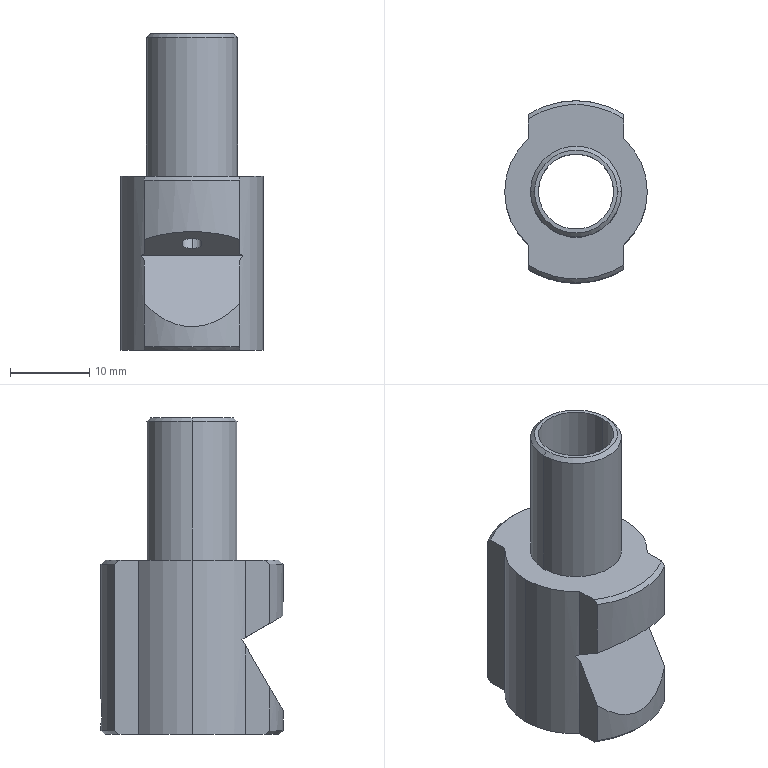Part | SolidWorks | features ICE 4, Chamfer 3, HoleWzd 3, Extrusion 1 | 1 solid | 42 faces | box 18 x 23 x 40 mm | volume 5124 mm3 | cylinder 18 | cone 12 | plane 12 | commonest cylinder face diameters 18 x3 23 x3 1.2 x2 2.5 x2 3.3 x2 9.5 x2
STEP:
#1=CARTESIAN_POINT('',(6.5,0.,0.5));
#2=VERTEX_POINT('',#1);
#3=CARTESIAN_POINT('',(-6.5,0.,0.5));
#4=VERTEX_POINT('',#3);
#5=CARTESIAN_POINT('',(0.,0.,0.5));
#6=DIRECTION('',(0.,0.,-1.));
#7=DIRECTION('',(1.,0.,0.));
#8=AXIS2_PLACEMENT_3D('',#5,#6,#7);
#9=CIRCLE('',#8,6.5);
#10=EDGE_CURVE('',#2,#4,#9,.T.);
#11=ORIENTED_EDGE('',*,*,#10,.F.);
#12=CARTESIAN_POINT('',(7.,0.,0.));
#13=VERTEX_POINT('',#12);
#14=CARTESIAN_POINT('',(6.5,0.,0.5));
#15=DIRECTION('',(0.7071,0.,-0.7071));
#16=VECTOR('',#15,1000.);
#17=LINE('',#14,#16);
#18=EDGE_CURVE('',#2,#13,#17,.T.);
#19=ORIENTED_EDGE('',*,*,#18,.T.);
#20=CARTESIAN_POINT('',(-7.,0.,0.));
#21=VERTEX_POINT('',#20);
#22=CARTESIAN_POINT('',(0.,0.,0.));
#23=DIRECTION('',(0.,0.,1.));
#24=DIRECTION('',(1.,0.,0.));
#25=AXIS2_PLACEMENT_3D('',#22,#23,#24);
#26=CIRCLE('',#25,7.);
#27=EDGE_CURVE('',#21,#13,#26,.T.);
#28=ORIENTED_EDGE('',*,*,#27,.F.);
#29=CARTESIAN_POINT('',(-6.5,0.,0.5));
#30=DIRECTION('',(-0.7071,0.,-0.7071));
#31=VECTOR('',#30,1000.);
#32=LINE('',#29,#31);
#33=EDGE_CURVE('',#4,#21,#32,.T.);
#34=ORIENTED_EDGE('',*,*,#33,.F.);
#35=EDGE_LOOP('',(#11,#19,#28,#34));
#36=FACE_OUTER_BOUND('',#35,.T.);
#37=CARTESIAN_POINT('',(0.,0.,0.5));
#38=DIRECTION('',(0.,0.,-1.));
#39=DIRECTION('',(-1.,0.,0.));
#40=AXIS2_PLACEMENT_3D('',#37,#38,#39);
#41=CONICAL_SURFACE('',#40,6.5,0.7854);
#42=ADVANCED_FACE('',(#36),#41,.F.);
#43=CARTESIAN_POINT('',(5.25,0.,40.));
#44=VERTEX_POINT('',#43);
#45=CARTESIAN_POINT('',(-5.25,0.,40.));
#46=VERTEX_POINT('',#45);
#47=CARTESIAN_POINT('',(0.,0.,40.));
#48=DIRECTION('',(0.,0.,1.));
#49=DIRECTION('',(1.,0.,0.));
#50=AXIS2_PLACEMENT_3D('',#47,#48,#49);
#51=CIRCLE('',#50,5.25);
#52=EDGE_CURVE('',#44,#46,#51,.T.);
#53=ORIENTED_EDGE('',*,*,#52,.F.);
#54=CARTESIAN_POINT('',(5.75,0.,39.5));
#55=VERTEX_POINT('',#54);
#56=CARTESIAN_POINT('',(5.25,0.,40.));
#57=DIRECTION('',(0.7071,0.,-0.7071));
#58=VECTOR('',#57,1000.);
#59=LINE('',#56,#58);
#60=EDGE_CURVE('',#44,#55,#59,.T.);
#61=ORIENTED_EDGE('',*,*,#60,.T.);
#62=CARTESIAN_POINT('',(-5.75,0.,39.5));
#63=VERTEX_POINT('',#62);
#64=CARTESIAN_POINT('',(0.,0.,39.5));
#65=DIRECTION('',(0.,0.,-1.));
#66=DIRECTION('',(1.,0.,0.));
#67=AXIS2_PLACEMENT_3D('',#64,#65,#66);
#68=CIRCLE('',#67,5.75);
#69=EDGE_CURVE('',#63,#55,#68,.T.);
#70=ORIENTED_EDGE('',*,*,#69,.F.);
#71=CARTESIAN_POINT('',(-5.25,0.,40.));
#72=DIRECTION('',(-0.7071,0.,-0.7071));
#73=VECTOR('',#72,1000.);
#74=LINE('',#71,#73);
#75=EDGE_CURVE('',#46,#63,#74,.T.);
#76=ORIENTED_EDGE('',*,*,#75,.F.);
#77=EDGE_LOOP('',(#53,#61,#70,#76));
#78=FACE_OUTER_BOUND('',#77,.T.);
#79=CARTESIAN_POINT('',(0.,0.,40.));
#80=DIRECTION('',(0.,0.,-1.));
#81=DIRECTION('',(-1.,0.,0.));
#82=AXIS2_PLACEMENT_3D('',#79,#80,#81);
#83=CONICAL_SURFACE('',#82,5.25,0.7854);
#84=ADVANCED_FACE('',(#78),#83,.T.);
#85=CARTESIAN_POINT('',(-6.,-6.708,22.));
#86=VERTEX_POINT('',#85);
#87=CARTESIAN_POINT('',(-9.,0.,22.));
#88=VERTEX_POINT('',#87);
#89=CARTESIAN_POINT('',(0.,0.,22.));
#90=DIRECTION('',(0.,0.,-1.));
#91=DIRECTION('',(1.,0.,0.));
#92=AXIS2_PLACEMENT_3D('',#89,#90,#91);
#93=CIRCLE('',#92,9.);
#94=EDGE_CURVE('',#86,#88,#93,.T.);
#95=ORIENTED_EDGE('',*,*,#94,.T.);
#96=CARTESIAN_POINT('',(-9.,0.,0.));
#97=VERTEX_POINT('',#96);
#98=CARTESIAN_POINT('',(-9.,0.,40.));
#99=DIRECTION('',(0.,0.,-1.));
#100=VECTOR('',#99,1000.);
#101=LINE('',#98,#100);
#102=EDGE_CURVE('',#88,#97,#101,.T.);
#103=ORIENTED_EDGE('',*,*,#102,.T.);
#104=CARTESIAN_POINT('',(-6.,-6.708,0.));
#105=VERTEX_POINT('',#104);
#106=CARTESIAN_POINT('',(0.,0.,0.));
#107=DIRECTION('',(0.,0.,1.));
#108=DIRECTION('',(-1.,0.,0.));
#109=AXIS2_PLACEMENT_3D('',#106,#107,#108);
#110=CIRCLE('',#109,9.);
#111=EDGE_CURVE('',#97,#105,#110,.T.);
#112=ORIENTED_EDGE('',*,*,#111,.T.);
#113=CARTESIAN_POINT('',(-6.,-6.708,11.3));
#114=VERTEX_POINT('',#113);
#115=CARTESIAN_POINT('',(-6.,-6.708,40.));
#116=DIRECTION('',(0.,0.,-1.));
#117=VECTOR('',#116,1000.);
#118=LINE('',#115,#117);
#119=EDGE_CURVE('',#114,#105,#118,.T.);
#120=ORIENTED_EDGE('',*,*,#119,.F.);
#121=CARTESIAN_POINT('',(-6.424,-6.304,12.));
#122=VERTEX_POINT('',#121);
#123=CARTESIAN_POINT('',(-6.424,-6.304,12.));
#124=CARTESIAN_POINT('',(-6.287,-6.443,11.759));
#125=CARTESIAN_POINT('',(-6.146,-6.578,11.525));
#126=CARTESIAN_POINT('',(-6.,-6.708,11.3));
#127=(BOUNDED_CURVE()B_SPLINE_CURVE(3,(#123,#124,#125,#126),.UNSPECIFIED.,.F.,.F.)B_SPLINE_CURVE_WITH_KNOTS((4,4),(5.488,5.553),.UNSPECIFIED.)CURVE()GEOMETRIC_REPRESENTATION_ITEM()RATIONAL_B_SPLINE_CURVE((1.,0.9996,0.9996,1.))REPRESENTATION_ITEM(''));
#128=EDGE_CURVE('',#122,#114,#127,.T.);
#129=ORIENTED_EDGE('',*,*,#128,.F.);
#130=CARTESIAN_POINT('',(-6.,-6.708,12.233));
#131=VERTEX_POINT('',#130);
#132=CARTESIAN_POINT('',(-6.,-6.708,12.233));
#133=CARTESIAN_POINT('',(-6.146,-6.578,12.158));
#134=CARTESIAN_POINT('',(-6.287,-6.443,12.08));
#135=CARTESIAN_POINT('',(-6.424,-6.304,12.));
#136=(BOUNDED_CURVE()B_SPLINE_CURVE(3,(#132,#133,#134,#135),.UNSPECIFIED.,.F.,.F.)B_SPLINE_CURVE_WITH_KNOTS((4,4),(3.871,3.936),.UNSPECIFIED.)CURVE()GEOMETRIC_REPRESENTATION_ITEM()RATIONAL_B_SPLINE_CURVE((1.,0.9996,0.9996,1.))REPRESENTATION_ITEM(''));
#137=EDGE_CURVE('',#131,#122,#136,.T.);
#138=ORIENTED_EDGE('',*,*,#137,.F.);
#139=CARTESIAN_POINT('',(-6.,-6.708,40.));
#140=DIRECTION('',(0.,0.,-1.));
#141=VECTOR('',#140,1000.);
#142=LINE('',#139,#141);
#143=EDGE_CURVE('',#86,#131,#142,.T.);
#144=ORIENTED_EDGE('',*,*,#143,.F.);
#145=EDGE_LOOP('',(#95,#103,#112,#120,#129,#138,#144));
#146=FACE_OUTER_BOUND('',#145,.T.);
#147=CARTESIAN_POINT('',(0.,0.,40.));
#148=DIRECTION('',(0.,0.,-1.));
#149=DIRECTION('',(-1.,0.,0.));
#150=AXIS2_PLACEMENT_3D('',#147,#148,#149);
#151=CYLINDRICAL_SURFACE('',#150,9.);
#152=ADVANCED_FACE('',(#146),#151,.T.);
#153=CARTESIAN_POINT('',(4.75,0.,16.));
#154=VERTEX_POINT('',#153);
#155=CARTESIAN_POINT('',(-4.75,0.,16.));
#156=VERTEX_POINT('',#155);
#157=CARTESIAN_POINT('',(0.,0.,16.));
#158=DIRECTION('',(0.,0.,-1.));
#159=DIRECTION('',(-1.,0.,0.));
#160=AXIS2_PLACEMENT_3D('',#157,#158,#159);
#161=CIRCLE('',#160,4.75);
#162=EDGE_CURVE('',#154,#156,#161,.T.);
#163=ORIENTED_EDGE('',*,*,#162,.F.);
#164=CARTESIAN_POINT('',(5.05,0.,8.));
#165=VERTEX_POINT('',#164);
#166=CARTESIAN_POINT('',(4.75,0.,16.));
#167=DIRECTION('',(0.03747,0.,-0.9993));
#168=VECTOR('',#167,1000.);
#169=LINE('',#166,#168);
#170=EDGE_CURVE('',#154,#165,#169,.T.);
#171=ORIENTED_EDGE('',*,*,#170,.T.);
#172=CARTESIAN_POINT('',(-5.05,0.,8.));
#173=VERTEX_POINT('',#172);
#174=CARTESIAN_POINT('',(0.,0.,8.));
#175=DIRECTION('',(0.,0.,1.));
#176=DIRECTION('',(-1.,0.,0.));
#177=AXIS2_PLACEMENT_3D('',#174,#175,#176);
#178=CIRCLE('',#177,5.05);
#179=EDGE_CURVE('',#173,#165,#178,.T.);
#180=ORIENTED_EDGE('',*,*,#179,.F.);
#181=CARTESIAN_POINT('',(-4.75,0.,16.));
#182=DIRECTION('',(-0.03747,0.,-0.9993));
#183=VECTOR('',#182,1000.);
#184=LINE('',#181,#183);
#185=EDGE_CURVE('',#156,#173,#184,.T.);
#186=ORIENTED_EDGE('',*,*,#185,.F.);
#187=EDGE_LOOP('',(#163,#171,#180,#186));
#188=FACE_OUTER_BOUND('',#187,.T.);
#189=CARTESIAN_POINT('',(0.,0.,16.));
#190=DIRECTION('',(0.,0.,-1.));
#191=DIRECTION('',(-1.,0.,0.));
#192=AXIS2_PLACEMENT_3D('',#189,#190,#191);
#193=CONICAL_SURFACE('',#192,4.75,0.03748);
#194=ADVANCED_FACE('',(#188),#193,.F.);
#195=CARTESIAN_POINT('',(0.,-7.734,18.022));
#196=VERTEX_POINT('',#195);
#197=CARTESIAN_POINT('',(0.,-5.569,16.772));
#198=VERTEX_POINT('',#197);
#199=CARTESIAN_POINT('',(0.,-6.652,17.397));
#200=DIRECTION('',(0.,-0.5,-0.866));
#201=DIRECTION('',(0.,0.866,-0.5));
#202=AXIS2_PLACEMENT_3D('',#199,#200,#201);
#203=CIRCLE('',#202,1.25);
#204=EDGE_CURVE('',#196,#198,#203,.T.);
#205=ORIENTED_EDGE('',*,*,#204,.F.);
#206=CARTESIAN_POINT('',(0.,-9.984,14.125));
#207=VERTEX_POINT('',#206);
#208=CARTESIAN_POINT('',(0.,-9.984,14.125));
#209=DIRECTION('',(0.,-0.5,-0.866));
#210=VECTOR('',#209,1000.);
#211=LINE('',#208,#210);
#212=EDGE_CURVE('',#196,#207,#211,.T.);
#213=ORIENTED_EDGE('',*,*,#212,.T.);
#214=CARTESIAN_POINT('',(0.,-7.819,12.875));
#215=VERTEX_POINT('',#214);
#216=CARTESIAN_POINT('',(0.,-8.902,13.5));
#217=DIRECTION('',(0.,-0.5,-0.866));
#218=DIRECTION('',(0.,0.866,-0.5));
#219=AXIS2_PLACEMENT_3D('',#216,#217,#218);
#220=CIRCLE('',#219,1.25);
#221=EDGE_CURVE('',#207,#215,#220,.T.);
#222=ORIENTED_EDGE('',*,*,#221,.T.);
#223=CARTESIAN_POINT('',(0.,-7.819,12.875));
#224=DIRECTION('',(0.,-0.5,-0.866));
#225=VECTOR('',#224,1000.);
#226=LINE('',#223,#225);
#227=EDGE_CURVE('',#198,#215,#226,.T.);
#228=ORIENTED_EDGE('',*,*,#227,.F.);
#229=EDGE_LOOP('',(#205,#213,#222,#228));
#230=FACE_OUTER_BOUND('',#229,.T.);
#231=CARTESIAN_POINT('',(0.,-8.902,13.5));
#232=DIRECTION('',(0.,-0.5,-0.866));
#233=DIRECTION('',(0.,0.866,-0.5));
#234=AXIS2_PLACEMENT_3D('',#231,#232,#233);
#235=CYLINDRICAL_SURFACE('',#234,1.25);
#236=ADVANCED_FACE('',(#230),#235,.F.);
#237=CARTESIAN_POINT('',(0.,-6.976,18.035));
#238=VERTEX_POINT('',#237);
#239=CARTESIAN_POINT('',(0.,-5.937,17.435));
#240=VERTEX_POINT('',#239);
#241=CARTESIAN_POINT('',(0.,-6.457,17.735));
#242=DIRECTION('',(0.,-0.5,-0.866));
#243=DIRECTION('',(0.,0.866,-0.5));
#244=AXIS2_PLACEMENT_3D('',#241,#242,#243);
#245=CIRCLE('',#244,0.6);
#246=EDGE_CURVE('',#238,#240,#245,.T.);
#247=ORIENTED_EDGE('',*,*,#246,.F.);
#248=CARTESIAN_POINT('',(0.,-7.734,18.022));
#249=DIRECTION('',(0.,-0.9998,-0.01745));
#250=VECTOR('',#249,1000.);
#251=LINE('',#248,#250);
#252=EDGE_CURVE('',#238,#196,#251,.T.);
#253=ORIENTED_EDGE('',*,*,#252,.T.);
#254=ORIENTED_EDGE('',*,*,#204,.T.);
#255=CARTESIAN_POINT('',(0.,-5.569,16.772));
#256=DIRECTION('',(0.,0.4848,-0.8746));
#257=VECTOR('',#256,1000.);
#258=LINE('',#255,#257);
#259=EDGE_CURVE('',#240,#198,#258,.T.);
#260=ORIENTED_EDGE('',*,*,#259,.F.);
#261=EDGE_LOOP('',(#247,#253,#254,#260));
#262=FACE_OUTER_BOUND('',#261,.T.);
#263=CARTESIAN_POINT('',(0.,-6.652,17.397));
#264=DIRECTION('',(0.,-0.5,-0.866));
#265=DIRECTION('',(0.,0.866,-0.5));
#266=AXIS2_PLACEMENT_3D('',#263,#264,#265);
#267=CONICAL_SURFACE('',#266,1.25,1.03);
#268=ADVANCED_FACE('',(#262),#267,.F.);
#269=CARTESIAN_POINT('',(0.,-4.75,19.491));
#270=VERTEX_POINT('',#269);
#271=CARTESIAN_POINT('',(0.,-4.75,21.891));
#272=VERTEX_POINT('',#271);
#273=CARTESIAN_POINT('',(0.,-4.75,19.491));
#274=CARTESIAN_POINT('',(-0.06183,-4.75,19.491));
#275=CARTESIAN_POINT('',(-0.121,-4.749,19.513));
#276=CARTESIAN_POINT('',(-0.2227,-4.745,19.581));
#277=CARTESIAN_POINT('',(-0.2659,-4.743,19.625));
#278=CARTESIAN_POINT('',(-0.3779,-4.736,19.768));
#279=CARTESIAN_POINT('',(-0.4309,-4.731,19.879));
#280=CARTESIAN_POINT('',(-0.5142,-4.722,20.106));
#281=CARTESIAN_POINT('',(-0.5439,-4.719,20.225));
#282=CARTESIAN_POINT('',(-0.585,-4.714,20.461));
#283=CARTESIAN_POINT('',(-0.5966,-4.712,20.581));
#284=CARTESIAN_POINT('',(-0.6049,-4.711,20.943));
#285=CARTESIAN_POINT('',(-0.5781,-4.715,21.187));
#286=CARTESIAN_POINT('',(-0.4528,-4.729,21.529));
#287=CARTESIAN_POINT('',(-0.3962,-4.734,21.64));
#288=CARTESIAN_POINT('',(-0.2756,-4.742,21.775));
#289=CARTESIAN_POINT('',(-0.2285,-4.745,21.816));
#290=CARTESIAN_POINT('',(-0.1218,-4.749,21.874));
#291=CARTESIAN_POINT('',(-0.06099,-4.75,21.891));
#292=CARTESIAN_POINT('',(0.,-4.75,21.891));
#293=B_SPLINE_CURVE_WITH_KNOTS('',3,(#273,#274,#275,#276,#277,#278,#279,#280,#281,#282,#283,#284,#285,#286,#287,#288,#289,#290,#291,#292),.UNSPECIFIED.,.F.,.F.,(4,2,2,2,2,2,2,2,2,4),(0.,0.0001825,0.0003651,0.0007301,0.001095,0.00146,0.00219,0.002556,0.002738,0.002921),.UNSPECIFIED.);
#294=EDGE_CURVE('',#270,#272,#293,.T.);
#295=ORIENTED_EDGE('',*,*,#294,.T.);
#296=CARTESIAN_POINT('',(0.,-9.422,13.8));
#297=DIRECTION('',(0.,-0.5,-0.866));
#298=VECTOR('',#297,1000.);
#299=LINE('',#296,#298);
#300=EDGE_CURVE('',#272,#238,#299,.T.);
#301=ORIENTED_EDGE('',*,*,#300,.T.);
#302=ORIENTED_EDGE('',*,*,#246,.T.);
#303=CARTESIAN_POINT('',(0.,-8.382,13.2));
#304=DIRECTION('',(0.,-0.5,-0.866));
#305=VECTOR('',#304,1000.);
#306=LINE('',#303,#305);
#307=EDGE_CURVE('',#270,#240,#306,.T.);
#308=ORIENTED_EDGE('',*,*,#307,.F.);
#309=EDGE_LOOP('',(#295,#301,#302,#308));
#310=FACE_OUTER_BOUND('',#309,.T.);
#311=CARTESIAN_POINT('',(0.,-8.902,13.5));
#312=DIRECTION('',(0.,-0.5,-0.866));
#313=DIRECTION('',(0.,0.866,-0.5));
#314=AXIS2_PLACEMENT_3D('',#311,#312,#313);
#315=CYLINDRICAL_SURFACE('',#314,0.6);
#316=ADVANCED_FACE('',(#310),#315,.F.);
#317=CARTESIAN_POINT('',(0.,11.5,4.65));
#318=VERTEX_POINT('',#317);
#319=CARTESIAN_POINT('',(0.,11.5,1.35));
#320=VERTEX_POINT('',#319);
#321=CARTESIAN_POINT('',(0.,11.5,4.65));
#322=CARTESIAN_POINT('',(-0.2155,11.5,4.65));
#323=CARTESIAN_POINT('',(-0.4328,11.494,4.607));
#324=CARTESIAN_POINT('',(-0.83,11.472,4.442));
#325=CARTESIAN_POINT('',(-1.014,11.456,4.319));
#326=CARTESIAN_POINT('',(-1.242,11.433,4.091));
#327=CARTESIAN_POINT('',(-1.312,11.425,4.007));
#328=CARTESIAN_POINT('',(-1.431,11.411,3.828));
#329=CARTESIAN_POINT('',(-1.482,11.404,3.733));
#330=CARTESIAN_POINT('',(-1.565,11.393,3.533));
#331=CARTESIAN_POINT('',(-1.597,11.389,3.429));
#332=CARTESIAN_POINT('',(-1.639,11.383,3.218));
#333=CARTESIAN_POINT('',(-1.65,11.381,3.11));
#334=CARTESIAN_POINT('',(-1.65,11.381,2.892));
#335=CARTESIAN_POINT('',(-1.639,11.383,2.785));
#336=CARTESIAN_POINT('',(-1.598,11.389,2.574));
#337=CARTESIAN_POINT('',(-1.566,11.393,2.469));
#338=CARTESIAN_POINT('',(-1.483,11.404,2.269));
#339=CARTESIAN_POINT('',(-1.433,11.411,2.174));
#340=CARTESIAN_POINT('',(-1.313,11.425,1.995));
#341=CARTESIAN_POINT('',(-1.243,11.433,1.91));
#342=CARTESIAN_POINT('',(-1.016,11.456,1.682));
#343=CARTESIAN_POINT('',(-0.8319,11.472,1.559));
#344=CARTESIAN_POINT('',(-0.4351,11.493,1.394));
#345=CARTESIAN_POINT('',(-0.2183,11.5,1.35));
#346=CARTESIAN_POINT('',(0.,11.5,1.35));
#347=B_SPLINE_CURVE_WITH_KNOTS('',3,(#321,#322,#323,#324,#325,#326,#327,#328,#329,#330,#331,#332,#333,#334,#335,#336,#337,#338,#339,#340,#341,#342,#343,#344,#345,#346),.UNSPECIFIED.,.F.,.F.,(4,2,2,2,2,2,2,2,2,2,2,2,4),(0.005165,0.005811,0.006456,0.006779,0.007102,0.007425,0.007747,0.00807,0.008393,0.008716,0.009038,0.009684,0.01033),.UNSPECIFIED.);
#348=EDGE_CURVE('',#318,#320,#347,.T.);
#349=ORIENTED_EDGE('',*,*,#348,.F.);
#350=CARTESIAN_POINT('',(0.,6.5,4.65));
#351=VERTEX_POINT('',#350);
#352=CARTESIAN_POINT('',(0.,0.,4.65));
#353=DIRECTION('',(0.,-1.,0.));
#354=VECTOR('',#353,1000.);
#355=LINE('',#352,#354);
#356=EDGE_CURVE('',#318,#351,#355,.T.);
#357=ORIENTED_EDGE('',*,*,#356,.T.);
#358=CARTESIAN_POINT('',(0.,6.5,1.35));
#359=VERTEX_POINT('',#358);
#360=CARTESIAN_POINT('',(0.,6.5,1.35));
#361=CARTESIAN_POINT('',(-0.1095,6.5,1.35));
#362=CARTESIAN_POINT('',(-0.2171,6.497,1.361));
#363=CARTESIAN_POINT('',(-0.4286,6.487,1.403));
#364=CARTESIAN_POINT('',(-0.5337,6.479,1.435));
#365=CARTESIAN_POINT('',(-0.7333,6.459,1.518));
#366=CARTESIAN_POINT('',(-0.8279,6.448,1.569));
#367=CARTESIAN_POINT('',(-1.007,6.422,1.688));
#368=CARTESIAN_POINT('',(-1.091,6.408,1.758));
#369=CARTESIAN_POINT('',(-1.319,6.367,1.985));
#370=CARTESIAN_POINT('',(-1.441,6.339,2.169));
#371=CARTESIAN_POINT('',(-1.606,6.299,2.565));
#372=CARTESIAN_POINT('',(-1.65,6.287,2.783));
#373=CARTESIAN_POINT('',(-1.65,6.287,3.107));
#374=CARTESIAN_POINT('',(-1.639,6.29,3.217));
#375=CARTESIAN_POINT('',(-1.597,6.301,3.429));
#376=CARTESIAN_POINT('',(-1.566,6.309,3.532));
#377=CARTESIAN_POINT('',(-1.441,6.339,3.833));
#378=CARTESIAN_POINT('',(-1.319,6.367,4.014));
#379=CARTESIAN_POINT('',(-1.09,6.408,4.243));
#380=CARTESIAN_POINT('',(-1.007,6.422,4.311));
#381=CARTESIAN_POINT('',(-0.8288,6.448,4.431));
#382=CARTESIAN_POINT('',(-0.7321,6.459,4.483));
#383=CARTESIAN_POINT('',(-0.533,6.479,4.565));
#384=CARTESIAN_POINT('',(-0.4301,6.487,4.597));
#385=CARTESIAN_POINT('',(-0.2175,6.497,4.639));
#386=CARTESIAN_POINT('',(-0.108,6.5,4.65));
#387=CARTESIAN_POINT('',(0.,6.5,4.65));
#388=B_SPLINE_CURVE_WITH_KNOTS('',3,(#360,#361,#362,#363,#364,#365,#366,#367,#368,#369,#370,#371,#372,#373,#374,#375,#376,#377,#378,#379,#380,#381,#382,#383,#384,#385,#386,#387),.UNSPECIFIED.,.F.,.F.,(4,2,2,2,2,2,2,2,2,2,2,2,2,4),(0.,0.0003237,0.0006475,0.0009712,0.001295,0.001942,0.00259,0.002914,0.003237,0.003885,0.004209,0.004532,0.004856,0.00518),.UNSPECIFIED.);
#389=EDGE_CURVE('',#359,#351,#388,.T.);
#390=ORIENTED_EDGE('',*,*,#389,.F.);
#391=CARTESIAN_POINT('',(0.,0.,1.35));
#392=DIRECTION('',(0.,-1.,0.));
#393=VECTOR('',#392,1000.);
#394=LINE('',#391,#393);
#395=EDGE_CURVE('',#320,#359,#394,.T.);
#396=ORIENTED_EDGE('',*,*,#395,.F.);
#397=EDGE_LOOP('',(#349,#357,#390,#396));
#398=FACE_OUTER_BOUND('',#397,.T.);
#399=CARTESIAN_POINT('',(0.,0.,3.));
#400=DIRECTION('',(0.,-1.,0.));
#401=DIRECTION('',(0.,0.,-1.));
#402=AXIS2_PLACEMENT_3D('',#399,#400,#401);
#403=CYLINDRICAL_SURFACE('',#402,1.65);
#404=ADVANCED_FACE('',(#398),#403,.F.);
#405=CARTESIAN_POINT('',(6.5,0.,8.));
#406=VERTEX_POINT('',#405);
#407=CARTESIAN_POINT('',(-6.5,0.,8.));
#408=VERTEX_POINT('',#407);
#409=CARTESIAN_POINT('',(0.,0.,8.));
#410=DIRECTION('',(0.,0.,-1.));
#411=DIRECTION('',(-1.,0.,0.));
#412=AXIS2_PLACEMENT_3D('',#409,#410,#411);
#413=CIRCLE('',#412,6.5);
#414=EDGE_CURVE('',#406,#408,#413,.T.);
#415=ORIENTED_EDGE('',*,*,#414,.F.);
#416=CARTESIAN_POINT('',(6.5,0.,8.));
#417=DIRECTION('',(0.,0.,-1.));
#418=VECTOR('',#417,1000.);
#419=LINE('',#416,#418);
#420=EDGE_CURVE('',#406,#2,#419,.T.);
#421=ORIENTED_EDGE('',*,*,#420,.T.);
#422=ORIENTED_EDGE('',*,*,#10,.T.);
#423=CARTESIAN_POINT('',(-6.5,0.,8.));
#424=DIRECTION('',(0.,0.,-1.));
#425=VECTOR('',#424,1000.);
#426=LINE('',#423,#425);
#427=EDGE_CURVE('',#408,#4,#426,.T.);
#428=ORIENTED_EDGE('',*,*,#427,.F.);
#429=EDGE_LOOP('',(#415,#421,#422,#428));
#430=FACE_OUTER_BOUND('',#429,.T.);
#431=CARTESIAN_POINT('',(0.,0.,8.));
#432=DIRECTION('',(0.,0.,-1.));
#433=DIRECTION('',(-1.,0.,0.));
#434=AXIS2_PLACEMENT_3D('',#431,#432,#433);
#435=CYLINDRICAL_SURFACE('',#434,6.5);
#436=ADVANCED_FACE('',(#430),#435,.F.);
#437=ORIENTED_EDGE('',*,*,#69,.T.);
#438=CARTESIAN_POINT('',(5.75,0.,22.));
#439=VERTEX_POINT('',#438);
#440=CARTESIAN_POINT('',(5.75,0.,40.));
#441=DIRECTION('',(0.,0.,-1.));
#442=VECTOR('',#441,1000.);
#443=LINE('',#440,#442);
#444=EDGE_CURVE('',#55,#439,#443,.T.);
#445=ORIENTED_EDGE('',*,*,#444,.T.);
#446=CARTESIAN_POINT('',(-5.75,0.,22.));
#447=VERTEX_POINT('',#446);
#448=CARTESIAN_POINT('',(0.,0.,22.));
#449=DIRECTION('',(0.,0.,1.));
#450=DIRECTION('',(1.,0.,0.));
#451=AXIS2_PLACEMENT_3D('',#448,#449,#450);
#452=CIRCLE('',#451,5.75);
#453=EDGE_CURVE('',#439,#447,#452,.T.);
#454=ORIENTED_EDGE('',*,*,#453,.T.);
#455=CARTESIAN_POINT('',(-5.75,0.,40.));
#456=DIRECTION('',(0.,0.,-1.));
#457=VECTOR('',#456,1000.);
#458=LINE('',#455,#457);
#459=EDGE_CURVE('',#63,#447,#458,.T.);
#460=ORIENTED_EDGE('',*,*,#459,.F.);
#461=EDGE_LOOP('',(#437,#445,#454,#460));
#462=FACE_OUTER_BOUND('',#461,.T.);
#463=CARTESIAN_POINT('',(0.,0.,40.));
#464=DIRECTION('',(0.,0.,-1.));
#465=DIRECTION('',(-1.,0.,0.));
#466=AXIS2_PLACEMENT_3D('',#463,#464,#465);
#467=CYLINDRICAL_SURFACE('',#466,5.75);
#468=ADVANCED_FACE('',(#462),#467,.T.);
#469=ORIENTED_EDGE('',*,*,#294,.F.);
#470=CARTESIAN_POINT('',(0.,-4.75,21.891));
#471=CARTESIAN_POINT('',(0.0611,-4.75,21.891));
#472=CARTESIAN_POINT('',(0.1215,-4.749,21.874));
#473=CARTESIAN_POINT('',(0.2288,-4.745,21.815));
#474=CARTESIAN_POINT('',(0.2755,-4.742,21.775));
#475=CARTESIAN_POINT('',(0.3971,-4.734,21.638));
#476=CARTESIAN_POINT('',(0.4532,-4.729,21.529));
#477=CARTESIAN_POINT('',(0.5366,-4.72,21.3));
#478=CARTESIAN_POINT('',(0.5631,-4.717,21.183));
#479=CARTESIAN_POINT('',(0.5961,-4.712,20.944));
#480=CARTESIAN_POINT('',(0.6021,-4.712,20.822));
#481=CARTESIAN_POINT('',(0.5966,-4.712,20.581));
#482=CARTESIAN_POINT('',(0.5851,-4.714,20.462));
#483=CARTESIAN_POINT('',(0.5441,-4.719,20.225));
#484=CARTESIAN_POINT('',(0.5143,-4.722,20.107));
#485=CARTESIAN_POINT('',(0.4308,-4.731,19.879));
#486=CARTESIAN_POINT('',(0.3778,-4.736,19.769));
#487=CARTESIAN_POINT('',(0.2669,-4.743,19.626));
#488=CARTESIAN_POINT('',(0.2234,-4.745,19.581));
#489=CARTESIAN_POINT('',(0.1213,-4.749,19.514));
#490=CARTESIAN_POINT('',(0.06195,-4.75,19.491));
#491=CARTESIAN_POINT('',(0.,-4.75,19.491));
#492=B_SPLINE_CURVE_WITH_KNOTS('',3,(#470,#471,#472,#473,#474,#475,#476,#477,#478,#479,#480,#481,#482,#483,#484,#485,#486,#487,#488,#489,#490,#491),.UNSPECIFIED.,.F.,.F.,(4,2,2,2,2,2,2,2,2,2,4),(0.002921,0.003103,0.003286,0.003652,0.004018,0.004384,0.004749,0.005115,0.005481,0.005664,0.005847),.UNSPECIFIED.);
#493=EDGE_CURVE('',#272,#270,#492,.T.);
#494=ORIENTED_EDGE('',*,*,#493,.F.);
#495=EDGE_LOOP('',(#469,#494));
#496=FACE_BOUND('',#495,.T.);
#497=CARTESIAN_POINT('',(-4.75,0.,40.));
#498=VERTEX_POINT('',#497);
#499=CARTESIAN_POINT('',(4.75,0.,40.));
#500=VERTEX_POINT('',#499);
#501=CARTESIAN_POINT('',(0.,0.,40.));
#502=DIRECTION('',(0.,0.,1.));
#503=DIRECTION('',(1.,0.,0.));
#504=AXIS2_PLACEMENT_3D('',#501,#502,#503);
#505=CIRCLE('',#504,4.75);
#506=EDGE_CURVE('',#498,#500,#505,.T.);
#507=ORIENTED_EDGE('',*,*,#506,.T.);
#508=CARTESIAN_POINT('',(4.75,0.,22.));
#509=DIRECTION('',(0.,0.,-1.));
#510=VECTOR('',#509,1000.);
#511=LINE('',#508,#510);
#512=EDGE_CURVE('',#500,#154,#511,.T.);
#513=ORIENTED_EDGE('',*,*,#512,.T.);
#514=ORIENTED_EDGE('',*,*,#162,.T.);
#515=CARTESIAN_POINT('',(-4.75,0.,22.));
#516=DIRECTION('',(0.,0.,-1.));
#517=VECTOR('',#516,1000.);
#518=LINE('',#515,#517);
#519=EDGE_CURVE('',#498,#156,#518,.T.);
#520=ORIENTED_EDGE('',*,*,#519,.F.);
#521=EDGE_LOOP('',(#507,#513,#514,#520));
#522=FACE_OUTER_BOUND('',#521,.T.);
#523=CARTESIAN_POINT('',(0.,0.,22.));
#524=DIRECTION('',(0.,0.,-1.));
#525=DIRECTION('',(-1.,0.,0.));
#526=AXIS2_PLACEMENT_3D('',#523,#524,#525);
#527=CYLINDRICAL_SURFACE('',#526,4.75);
#528=ADVANCED_FACE('',(#496,#522),#527,.F.);
#529=CARTESIAN_POINT('',(-6.,-9.811,0.5));
#530=VERTEX_POINT('',#529);
#531=CARTESIAN_POINT('',(6.,-9.811,0.5));
#532=VERTEX_POINT('',#531);
#533=CARTESIAN_POINT('',(0.,0.,0.5));
#534=DIRECTION('',(0.,0.,1.));
#535=DIRECTION('',(1.,0.,0.));
#536=AXIS2_PLACEMENT_3D('',#533,#534,#535);
#537=CIRCLE('',#536,11.5);
#538=EDGE_CURVE('',#530,#532,#537,.T.);
#539=ORIENTED_EDGE('',*,*,#538,.T.);
#540=CARTESIAN_POINT('',(6.,-9.811,5.926));
#541=VERTEX_POINT('',#540);
#542=CARTESIAN_POINT('',(6.,-9.811,40.));
#543=DIRECTION('',(0.,0.,-1.));
#544=VECTOR('',#543,1000.);
#545=LINE('',#542,#544);
#546=EDGE_CURVE('',#541,#532,#545,.T.);
#547=ORIENTED_EDGE('',*,*,#546,.F.);
#548=CARTESIAN_POINT('',(-6.,-9.811,5.926));
#549=VERTEX_POINT('',#548);
#550=CARTESIAN_POINT('',(6.,-9.811,5.926));
#551=CARTESIAN_POINT('',(2.217,-12.124,1.919));
#552=CARTESIAN_POINT('',(-2.217,-12.124,1.919));
#553=CARTESIAN_POINT('',(-6.,-9.811,5.926));
#554=(BOUNDED_CURVE()B_SPLINE_CURVE(3,(#550,#551,#552,#553),.UNSPECIFIED.,.F.,.F.)B_SPLINE_CURVE_WITH_KNOTS((4,4),(5.734,6.832),.UNSPECIFIED.)CURVE()GEOMETRIC_REPRESENTATION_ITEM()RATIONAL_B_SPLINE_CURVE((1.,0.9021,0.9021,1.))REPRESENTATION_ITEM(''));
#555=EDGE_CURVE('',#541,#549,#554,.T.);
#556=ORIENTED_EDGE('',*,*,#555,.T.);
#557=CARTESIAN_POINT('',(-6.,-9.811,40.));
#558=DIRECTION('',(0.,0.,-1.));
#559=VECTOR('',#558,1000.);
#560=LINE('',#557,#559);
#561=EDGE_CURVE('',#549,#530,#560,.T.);
#562=ORIENTED_EDGE('',*,*,#561,.T.);
#563=EDGE_LOOP('',(#539,#547,#556,#562));
#564=FACE_OUTER_BOUND('',#563,.T.);
#565=CARTESIAN_POINT('',(0.,0.,22.));
#566=DIRECTION('',(0.,0.,-1.));
#567=DIRECTION('',(-1.,0.,0.));
#568=AXIS2_PLACEMENT_3D('',#565,#566,#567);
#569=CYLINDRICAL_SURFACE('',#568,11.5);
#570=ADVANCED_FACE('',(#564),#569,.T.);
#571=CARTESIAN_POINT('',(-6.,-9.811,14.025));
#572=VERTEX_POINT('',#571);
#573=CARTESIAN_POINT('',(6.,-9.811,14.025));
#574=VERTEX_POINT('',#573);
#575=CARTESIAN_POINT('',(-6.,-9.811,14.025));
#576=CARTESIAN_POINT('',(-2.217,-12.124,15.36));
#577=CARTESIAN_POINT('',(2.217,-12.124,15.36));
#578=CARTESIAN_POINT('',(6.,-9.811,14.025));
#579=(BOUNDED_CURVE()B_SPLINE_CURVE(3,(#575,#576,#577,#578),.UNSPECIFIED.,.F.,.F.)B_SPLINE_CURVE_WITH_KNOTS((4,4),(2.593,3.69),.UNSPECIFIED.)CURVE()GEOMETRIC_REPRESENTATION_ITEM()RATIONAL_B_SPLINE_CURVE((1.,0.9021,0.9021,1.))REPRESENTATION_ITEM(''));
#580=EDGE_CURVE('',#572,#574,#579,.T.);
#581=ORIENTED_EDGE('',*,*,#580,.T.);
#582=CARTESIAN_POINT('',(6.,-9.811,21.5));
#583=VERTEX_POINT('',#582);
#584=CARTESIAN_POINT('',(6.,-9.811,40.));
#585=DIRECTION('',(0.,0.,-1.));
#586=VECTOR('',#585,1000.);
#587=LINE('',#584,#586);
#588=EDGE_CURVE('',#583,#574,#587,.T.);
#589=ORIENTED_EDGE('',*,*,#588,.F.);
#590=CARTESIAN_POINT('',(-6.,-9.811,21.5));
#591=VERTEX_POINT('',#590);
#592=CARTESIAN_POINT('',(0.,0.,21.5));
#593=DIRECTION('',(0.,0.,-1.));
#594=DIRECTION('',(1.,0.,0.));
#595=AXIS2_PLACEMENT_3D('',#592,#593,#594);
#596=CIRCLE('',#595,11.5);
#597=EDGE_CURVE('',#583,#591,#596,.T.);
#598=ORIENTED_EDGE('',*,*,#597,.T.);
#599=CARTESIAN_POINT('',(-6.,-9.811,40.));
#600=DIRECTION('',(0.,0.,-1.));
#601=VECTOR('',#600,1000.);
#602=LINE('',#599,#601);
#603=EDGE_CURVE('',#591,#572,#602,.T.);
#604=ORIENTED_EDGE('',*,*,#603,.T.);
#605=EDGE_LOOP('',(#581,#589,#598,#604));
#606=FACE_OUTER_BOUND('',#605,.T.);
#607=CARTESIAN_POINT('',(0.,0.,22.));
#608=DIRECTION('',(0.,0.,-1.));
#609=DIRECTION('',(-1.,0.,0.));
#610=AXIS2_PLACEMENT_3D('',#607,#608,#609);
#611=CYLINDRICAL_SURFACE('',#610,11.5);
#612=ADVANCED_FACE('',(#606),#611,.T.);
#613=CARTESIAN_POINT('',(6.,-9.22,22.));
#614=VERTEX_POINT('',#613);
#615=CARTESIAN_POINT('',(6.,-9.22,22.));
#616=CARTESIAN_POINT('',(6.,-9.417,21.834));
#617=CARTESIAN_POINT('',(6.,-9.614,21.667));
#618=CARTESIAN_POINT('',(6.,-9.811,21.5));
#619=B_SPLINE_CURVE_WITH_KNOTS('',3,(#615,#616,#617,#618),.UNSPECIFIED.,.F.,.F.,(4,4),(0.005475,0.006248),.UNSPECIFIED.);
#620=EDGE_CURVE('',#614,#583,#619,.T.);
#621=ORIENTED_EDGE('',*,*,#620,.F.);
#622=CARTESIAN_POINT('',(-6.,-9.22,22.));
#623=VERTEX_POINT('',#622);
#624=CARTESIAN_POINT('',(0.,0.,22.));
#625=DIRECTION('',(0.,0.,1.));
#626=DIRECTION('',(1.,0.,0.));
#627=AXIS2_PLACEMENT_3D('',#624,#625,#626);
#628=CIRCLE('',#627,11.);
#629=EDGE_CURVE('',#623,#614,#628,.T.);
#630=ORIENTED_EDGE('',*,*,#629,.F.);
#631=CARTESIAN_POINT('',(-6.,-9.811,21.5));
#632=CARTESIAN_POINT('',(-6.,-9.614,21.667));
#633=CARTESIAN_POINT('',(-6.,-9.417,21.834));
#634=CARTESIAN_POINT('',(-6.,-9.22,22.));
#635=B_SPLINE_CURVE_WITH_KNOTS('',3,(#631,#632,#633,#634),.UNSPECIFIED.,.F.,.F.,(4,4),(0.005327,0.006101),.UNSPECIFIED.);
#636=EDGE_CURVE('',#591,#623,#635,.T.);
#637=ORIENTED_EDGE('',*,*,#636,.F.);
#638=ORIENTED_EDGE('',*,*,#597,.F.);
#639=EDGE_LOOP('',(#621,#630,#637,#638));
#640=FACE_OUTER_BOUND('',#639,.T.);
#641=CARTESIAN_POINT('',(0.,0.,22.));
#642=DIRECTION('',(0.,0.,-1.));
#643=DIRECTION('',(-1.,0.,0.));
#644=AXIS2_PLACEMENT_3D('',#641,#642,#643);
#645=CONICAL_SURFACE('',#644,11.,0.7854);
#646=ADVANCED_FACE('',(#640),#645,.T.);
#647=CARTESIAN_POINT('',(6.,-9.22,0.));
#648=VERTEX_POINT('',#647);
#649=CARTESIAN_POINT('',(6.,-9.811,0.5));
#650=CARTESIAN_POINT('',(6.,-9.614,0.3325));
#651=CARTESIAN_POINT('',(6.,-9.417,0.1658));
#652=CARTESIAN_POINT('',(6.,-9.22,0.));
#653=B_SPLINE_CURVE_WITH_KNOTS('',3,(#649,#650,#651,#652),.UNSPECIFIED.,.F.,.F.,(4,4),(0.005327,0.006101),.UNSPECIFIED.);
#654=EDGE_CURVE('',#532,#648,#653,.T.);
#655=ORIENTED_EDGE('',*,*,#654,.F.);
#656=ORIENTED_EDGE('',*,*,#538,.F.);
#657=CARTESIAN_POINT('',(-6.,-9.22,0.));
#658=VERTEX_POINT('',#657);
#659=CARTESIAN_POINT('',(-6.,-9.22,0.));
#660=CARTESIAN_POINT('',(-6.,-9.417,0.1658));
#661=CARTESIAN_POINT('',(-6.,-9.614,0.3325));
#662=CARTESIAN_POINT('',(-6.,-9.811,0.5));
#663=B_SPLINE_CURVE_WITH_KNOTS('',3,(#659,#660,#661,#662),.UNSPECIFIED.,.F.,.F.,(4,4),(0.005475,0.006248),.UNSPECIFIED.);
#664=EDGE_CURVE('',#658,#530,#663,.T.);
#665=ORIENTED_EDGE('',*,*,#664,.F.);
#666=CARTESIAN_POINT('',(0.,0.,0.));
#667=DIRECTION('',(0.,0.,-1.));
#668=DIRECTION('',(1.,0.,0.));
#669=AXIS2_PLACEMENT_3D('',#666,#667,#668);
#670=CIRCLE('',#669,11.);
#671=EDGE_CURVE('',#648,#658,#670,.T.);
#672=ORIENTED_EDGE('',*,*,#671,.F.);
#673=EDGE_LOOP('',(#655,#656,#665,#672));
#674=FACE_OUTER_BOUND('',#673,.T.);
#675=CARTESIAN_POINT('',(0.,0.,0.5));
#676=DIRECTION('',(0.,0.,1.));
#677=DIRECTION('',(1.,0.,0.));
#678=AXIS2_PLACEMENT_3D('',#675,#676,#677);
#679=CONICAL_SURFACE('',#678,11.5,0.7854);
#680=ADVANCED_FACE('',(#674),#679,.T.);
#681=CARTESIAN_POINT('',(0.,-8.902,13.5));
#682=DIRECTION('',(0.,-0.5,-0.866));
#683=DIRECTION('',(0.,0.866,-0.5));
#684=AXIS2_PLACEMENT_3D('',#681,#682,#683);
#685=CIRCLE('',#684,1.25);
#686=EDGE_CURVE('',#215,#207,#685,.T.);
#687=ORIENTED_EDGE('',*,*,#686,.F.);
#688=ORIENTED_EDGE('',*,*,#221,.F.);
#689=EDGE_LOOP('',(#687,#688));
#690=FACE_BOUND('',#689,.T.);
#691=CARTESIAN_POINT('',(6.424,-6.304,12.));
#692=VERTEX_POINT('',#691);
#693=CARTESIAN_POINT('',(-11.5,-6.304,12.));
#694=DIRECTION('',(1.,0.,0.));
#695=VECTOR('',#694,1000.);
#696=LINE('',#693,#695);
#697=EDGE_CURVE('',#122,#692,#696,.T.);
#698=ORIENTED_EDGE('',*,*,#697,.T.);
#699=CARTESIAN_POINT('',(6.,-6.708,12.233));
#700=VERTEX_POINT('',#699);
#701=CARTESIAN_POINT('',(6.424,-6.304,12.));
#702=CARTESIAN_POINT('',(6.287,-6.443,12.08));
#703=CARTESIAN_POINT('',(6.146,-6.578,12.158));
#704=CARTESIAN_POINT('',(6.,-6.708,12.233));
#705=(BOUNDED_CURVE()B_SPLINE_CURVE(3,(#701,#702,#703,#704),.UNSPECIFIED.,.F.,.F.)B_SPLINE_CURVE_WITH_KNOTS((4,4),(2.347,2.412),.UNSPECIFIED.)CURVE()GEOMETRIC_REPRESENTATION_ITEM()RATIONAL_B_SPLINE_CURVE((1.,0.9996,0.9996,1.))REPRESENTATION_ITEM(''));
#706=EDGE_CURVE('',#692,#700,#705,.T.);
#707=ORIENTED_EDGE('',*,*,#706,.T.);
#708=CARTESIAN_POINT('',(6.,-11.5,15.));
#709=DIRECTION('',(0.,-0.866,0.5));
#710=VECTOR('',#709,1000.);
#711=LINE('',#708,#710);
#712=EDGE_CURVE('',#700,#574,#711,.T.);
#713=ORIENTED_EDGE('',*,*,#712,.T.);
#714=ORIENTED_EDGE('',*,*,#580,.F.);
#715=CARTESIAN_POINT('',(-6.,-11.5,15.));
#716=DIRECTION('',(0.,0.866,-0.5));
#717=VECTOR('',#716,1000.);
#718=LINE('',#715,#717);
#719=EDGE_CURVE('',#572,#131,#718,.T.);
#720=ORIENTED_EDGE('',*,*,#719,.T.);
#721=ORIENTED_EDGE('',*,*,#137,.T.);
#722=EDGE_LOOP('',(#698,#707,#713,#714,#720,#721));
#723=FACE_OUTER_BOUND('',#722,.T.);
#724=CARTESIAN_POINT('',(-11.5,-11.5,15.));
#725=DIRECTION('',(0.,0.5,0.866));
#726=DIRECTION('',(0.,-0.866,0.5));
#727=AXIS2_PLACEMENT_3D('',#724,#725,#726);
#728=PLANE('',#727);
#729=ADVANCED_FACE('',(#690,#723),#728,.F.);
#730=ORIENTED_EDGE('',*,*,#512,.F.);
#731=CARTESIAN_POINT('',(0.,0.,40.));
#732=DIRECTION('',(0.,0.,1.));
#733=DIRECTION('',(1.,0.,0.));
#734=AXIS2_PLACEMENT_3D('',#731,#732,#733);
#735=CIRCLE('',#734,4.75);
#736=EDGE_CURVE('',#500,#498,#735,.T.);
#737=ORIENTED_EDGE('',*,*,#736,.T.);
#738=ORIENTED_EDGE('',*,*,#519,.T.);
#739=CARTESIAN_POINT('',(0.,0.,16.));
#740=DIRECTION('',(0.,0.,-1.));
#741=DIRECTION('',(-1.,0.,0.));
#742=AXIS2_PLACEMENT_3D('',#739,#740,#741);
#743=CIRCLE('',#742,4.75);
#744=EDGE_CURVE('',#156,#154,#743,.T.);
#745=ORIENTED_EDGE('',*,*,#744,.T.);
#746=EDGE_LOOP('',(#730,#737,#738,#745));
#747=FACE_OUTER_BOUND('',#746,.T.);
#748=CARTESIAN_POINT('',(0.,0.,22.));
#749=DIRECTION('',(0.,0.,-1.));
#750=DIRECTION('',(-1.,0.,0.));
#751=AXIS2_PLACEMENT_3D('',#748,#749,#750);
#752=CYLINDRICAL_SURFACE('',#751,4.75);
#753=ADVANCED_FACE('',(#747),#752,.F.);
#754=CARTESIAN_POINT('',(6.,-6.708,22.));
#755=VERTEX_POINT('',#754);
#756=CARTESIAN_POINT('',(6.,0.,22.));
#757=DIRECTION('',(0.,-1.,0.));
#758=VECTOR('',#757,1000.);
#759=LINE('',#756,#758);
#760=EDGE_CURVE('',#755,#614,#759,.T.);
#761=ORIENTED_EDGE('',*,*,#760,.F.);
#762=CARTESIAN_POINT('',(6.,6.708,22.));
#763=VERTEX_POINT('',#762);
#764=CARTESIAN_POINT('',(0.,0.,22.));
#765=DIRECTION('',(0.,0.,-1.));
#766=DIRECTION('',(1.,0.,0.));
#767=AXIS2_PLACEMENT_3D('',#764,#765,#766);
#768=CIRCLE('',#767,9.);
#769=EDGE_CURVE('',#763,#755,#768,.T.);
#770=ORIENTED_EDGE('',*,*,#769,.F.);
#771=CARTESIAN_POINT('',(6.,9.22,22.));
#772=VERTEX_POINT('',#771);
#773=CARTESIAN_POINT('',(6.,0.,22.));
#774=DIRECTION('',(0.,-1.,0.));
#775=VECTOR('',#774,1000.);
#776=LINE('',#773,#775);
#777=EDGE_CURVE('',#772,#763,#776,.T.);
#778=ORIENTED_EDGE('',*,*,#777,.F.);
#779=CARTESIAN_POINT('',(-6.,9.22,22.));
#780=VERTEX_POINT('',#779);
#781=CARTESIAN_POINT('',(0.,0.,22.));
#782=DIRECTION('',(0.,0.,1.));
#783=DIRECTION('',(1.,0.,0.));
#784=AXIS2_PLACEMENT_3D('',#781,#782,#783);
#785=CIRCLE('',#784,11.);
#786=EDGE_CURVE('',#772,#780,#785,.T.);
#787=ORIENTED_EDGE('',*,*,#786,.T.);
#788=CARTESIAN_POINT('',(-6.,6.708,22.));
#789=VERTEX_POINT('',#788);
#790=CARTESIAN_POINT('',(-6.,0.,22.));
#791=DIRECTION('',(0.,1.,0.));
#792=VECTOR('',#791,1000.);
#793=LINE('',#790,#792);
#794=EDGE_CURVE('',#789,#780,#793,.T.);
#795=ORIENTED_EDGE('',*,*,#794,.F.);
#796=CARTESIAN_POINT('',(0.,0.,22.));
#797=DIRECTION('',(0.,0.,-1.));
#798=DIRECTION('',(1.,0.,0.));
#799=AXIS2_PLACEMENT_3D('',#796,#797,#798);
#800=CIRCLE('',#799,9.);
#801=EDGE_CURVE('',#88,#789,#800,.T.);
#802=ORIENTED_EDGE('',*,*,#801,.F.);
#803=ORIENTED_EDGE('',*,*,#94,.F.);
#804=CARTESIAN_POINT('',(-6.,0.,22.));
#805=DIRECTION('',(0.,1.,0.));
#806=VECTOR('',#805,1000.);
#807=LINE('',#804,#806);
#808=EDGE_CURVE('',#623,#86,#807,.T.);
#809=ORIENTED_EDGE('',*,*,#808,.F.);
#810=ORIENTED_EDGE('',*,*,#629,.T.);
#811=EDGE_LOOP('',(#761,#770,#778,#787,#795,#802,#803,#809,#810));
#812=FACE_OUTER_BOUND('',#811,.T.);
#813=CARTESIAN_POINT('',(0.,0.,22.));
#814=DIRECTION('',(0.,0.,1.));
#815=DIRECTION('',(1.,0.,0.));
#816=AXIS2_PLACEMENT_3D('',#813,#814,#815);
#817=CIRCLE('',#816,5.75);
#818=EDGE_CURVE('',#447,#439,#817,.T.);
#819=ORIENTED_EDGE('',*,*,#818,.F.);
#820=ORIENTED_EDGE('',*,*,#453,.F.);
#821=EDGE_LOOP('',(#819,#820));
#822=FACE_BOUND('',#821,.T.);
#823=CARTESIAN_POINT('',(0.,0.,22.));
#824=DIRECTION('',(0.,0.,1.));
#825=DIRECTION('',(1.,0.,0.));
#826=AXIS2_PLACEMENT_3D('',#823,#824,#825);
#827=PLANE('',#826);
#828=ADVANCED_FACE('',(#812,#822),#827,.T.);
#829=ORIENTED_EDGE('',*,*,#27,.T.);
#830=CARTESIAN_POINT('',(0.,0.,0.));
#831=DIRECTION('',(0.,0.,1.));
#832=DIRECTION('',(1.,0.,0.));
#833=AXIS2_PLACEMENT_3D('',#830,#831,#832);
#834=CIRCLE('',#833,7.);
#835=EDGE_CURVE('',#13,#21,#834,.T.);
#836=ORIENTED_EDGE('',*,*,#835,.T.);
#837=EDGE_LOOP('',(#829,#836));
#838=FACE_BOUND('',#837,.T.);
#839=CARTESIAN_POINT('',(6.,-6.708,0.));
#840=VERTEX_POINT('',#839);
#841=CARTESIAN_POINT('',(6.,6.708,0.));
#842=VERTEX_POINT('',#841);
#843=CARTESIAN_POINT('',(0.,0.,0.));
#844=DIRECTION('',(0.,0.,1.));
#845=DIRECTION('',(-1.,0.,0.));
#846=AXIS2_PLACEMENT_3D('',#843,#844,#845);
#847=CIRCLE('',#846,9.);
#848=EDGE_CURVE('',#840,#842,#847,.T.);
#849=ORIENTED_EDGE('',*,*,#848,.F.);
#850=CARTESIAN_POINT('',(6.,-6.708,0.));
#851=DIRECTION('',(0.,1.,0.));
#852=VECTOR('',#851,1000.);
#853=LINE('',#850,#852);
#854=EDGE_CURVE('',#648,#840,#853,.T.);
#855=ORIENTED_EDGE('',*,*,#854,.F.);
#856=ORIENTED_EDGE('',*,*,#671,.T.);
#857=CARTESIAN_POINT('',(-6.,-6.708,0.));
#858=DIRECTION('',(0.,-1.,0.));
#859=VECTOR('',#858,1000.);
#860=LINE('',#857,#859);
#861=EDGE_CURVE('',#105,#658,#860,.T.);
#862=ORIENTED_EDGE('',*,*,#861,.F.);
#863=ORIENTED_EDGE('',*,*,#111,.F.);
#864=CARTESIAN_POINT('',(-6.,6.708,0.));
#865=VERTEX_POINT('',#864);
#866=CARTESIAN_POINT('',(0.,0.,0.));
#867=DIRECTION('',(0.,0.,1.));
#868=DIRECTION('',(-1.,0.,0.));
#869=AXIS2_PLACEMENT_3D('',#866,#867,#868);
#870=CIRCLE('',#869,9.);
#871=EDGE_CURVE('',#865,#97,#870,.T.);
#872=ORIENTED_EDGE('',*,*,#871,.F.);
#873=CARTESIAN_POINT('',(-6.,9.22,0.));
#874=VERTEX_POINT('',#873);
#875=CARTESIAN_POINT('',(-6.,9.811,0.));
#876=DIRECTION('',(0.,-1.,0.));
#877=VECTOR('',#876,1000.);
#878=LINE('',#875,#877);
#879=EDGE_CURVE('',#874,#865,#878,.T.);
#880=ORIENTED_EDGE('',*,*,#879,.F.);
#881=CARTESIAN_POINT('',(6.,9.22,0.));
#882=VERTEX_POINT('',#881);
#883=CARTESIAN_POINT('',(0.,0.,0.));
#884=DIRECTION('',(0.,0.,-1.));
#885=DIRECTION('',(1.,0.,0.));
#886=AXIS2_PLACEMENT_3D('',#883,#884,#885);
#887=CIRCLE('',#886,11.);
#888=EDGE_CURVE('',#874,#882,#887,.T.);
#889=ORIENTED_EDGE('',*,*,#888,.T.);
#890=CARTESIAN_POINT('',(6.,9.811,0.));
#891=DIRECTION('',(0.,1.,0.));
#892=VECTOR('',#891,1000.);
#893=LINE('',#890,#892);
#894=EDGE_CURVE('',#842,#882,#893,.T.);
#895=ORIENTED_EDGE('',*,*,#894,.F.);
#896=EDGE_LOOP('',(#849,#855,#856,#862,#863,#872,#880,#889,#895));
#897=FACE_OUTER_BOUND('',#896,.T.);
#898=CARTESIAN_POINT('',(0.,0.,0.));
#899=DIRECTION('',(0.,0.,1.));
#900=DIRECTION('',(1.,0.,0.));
#901=AXIS2_PLACEMENT_3D('',#898,#899,#900);
#902=PLANE('',#901);
#903=ADVANCED_FACE('',(#838,#897),#902,.F.);
#904=CARTESIAN_POINT('',(-6.,9.811,21.5));
#905=VERTEX_POINT('',#904);
#906=CARTESIAN_POINT('',(6.,9.811,21.5));
#907=VERTEX_POINT('',#906);
#908=CARTESIAN_POINT('',(0.,0.,21.5));
#909=DIRECTION('',(0.,0.,-1.));
#910=DIRECTION('',(1.,0.,0.));
#911=AXIS2_PLACEMENT_3D('',#908,#909,#910);
#912=CIRCLE('',#911,11.5);
#913=EDGE_CURVE('',#905,#907,#912,.T.);
#914=ORIENTED_EDGE('',*,*,#913,.T.);
#915=CARTESIAN_POINT('',(6.,9.811,0.5));
#916=VERTEX_POINT('',#915);
#917=CARTESIAN_POINT('',(6.,9.811,40.));
#918=DIRECTION('',(0.,0.,-1.));
#919=VECTOR('',#918,1000.);
#920=LINE('',#917,#919);
#921=EDGE_CURVE('',#907,#916,#920,.T.);
#922=ORIENTED_EDGE('',*,*,#921,.T.);
#923=CARTESIAN_POINT('',(-6.,9.811,0.5));
#924=VERTEX_POINT('',#923);
#925=CARTESIAN_POINT('',(0.,0.,0.5));
#926=DIRECTION('',(0.,0.,1.));
#927=DIRECTION('',(1.,0.,0.));
#928=AXIS2_PLACEMENT_3D('',#925,#926,#927);
#929=CIRCLE('',#928,11.5);
#930=EDGE_CURVE('',#916,#924,#929,.T.);
#931=ORIENTED_EDGE('',*,*,#930,.T.);
#932=CARTESIAN_POINT('',(-6.,9.811,40.));
#933=DIRECTION('',(0.,0.,-1.));
#934=VECTOR('',#933,1000.);
#935=LINE('',#932,#934);
#936=EDGE_CURVE('',#905,#924,#935,.T.);
#937=ORIENTED_EDGE('',*,*,#936,.F.);
#938=EDGE_LOOP('',(#914,#922,#931,#937));
#939=FACE_OUTER_BOUND('',#938,.T.);
#940=CARTESIAN_POINT('',(0.,11.5,1.35));
#941=CARTESIAN_POINT('',(0.1092,11.5,1.35));
#942=CARTESIAN_POINT('',(0.2165,11.498,1.361));
#943=CARTESIAN_POINT('',(0.4276,11.493,1.403));
#944=CARTESIAN_POINT('',(0.5325,11.488,1.435));
#945=CARTESIAN_POINT('',(0.7322,11.477,1.517));
#946=CARTESIAN_POINT('',(0.827,11.471,1.568));
#947=CARTESIAN_POINT('',(1.006,11.456,1.688));
#948=CARTESIAN_POINT('',(1.091,11.448,1.757));
#949=CARTESIAN_POINT('',(1.319,11.425,1.986));
#950=CARTESIAN_POINT('',(1.442,11.41,2.169));
#951=CARTESIAN_POINT('',(1.606,11.388,2.566));
#952=CARTESIAN_POINT('',(1.65,11.381,2.784));
#953=CARTESIAN_POINT('',(1.65,11.381,3.107));
#954=CARTESIAN_POINT('',(1.639,11.383,3.217));
#955=CARTESIAN_POINT('',(1.597,11.389,3.428));
#956=CARTESIAN_POINT('',(1.566,11.393,3.531));
#957=CARTESIAN_POINT('',(1.483,11.404,3.731));
#958=CARTESIAN_POINT('',(1.431,11.411,3.828));
#959=CARTESIAN_POINT('',(1.312,11.425,4.006));
#960=CARTESIAN_POINT('',(1.244,11.433,4.09));
#961=CARTESIAN_POINT('',(1.09,11.448,4.244));
#962=CARTESIAN_POINT('',(1.007,11.456,4.312));
#963=CARTESIAN_POINT('',(0.8281,11.47,4.431));
#964=CARTESIAN_POINT('',(0.7316,11.477,4.483));
#965=CARTESIAN_POINT('',(0.5318,11.488,4.566));
#966=CARTESIAN_POINT('',(0.429,11.492,4.597));
#967=CARTESIAN_POINT('',(0.2172,11.498,4.639));
#968=CARTESIAN_POINT('',(0.1078,11.5,4.65));
#969=CARTESIAN_POINT('',(0.,11.5,4.65));
#970=B_SPLINE_CURVE_WITH_KNOTS('',3,(#940,#941,#942,#943,#944,#945,#946,#947,#948,#949,#950,#951,#952,#953,#954,#955,#956,#957,#958,#959,#960,#961,#962,#963,#964,#965,#966,#967,#968,#969),.UNSPECIFIED.,.F.,.F.,(4,2,2,2,2,2,2,2,2,2,2,2,2,2,4),(0.,0.0003228,0.0006457,0.0009685,0.001291,0.001937,0.002583,0.002905,0.003228,0.003551,0.003874,0.004197,0.00452,0.004842,0.005165),.UNSPECIFIED.);
#971=EDGE_CURVE('',#320,#318,#970,.T.);
#972=ORIENTED_EDGE('',*,*,#971,.T.);
#973=ORIENTED_EDGE('',*,*,#348,.T.);
#974=EDGE_LOOP('',(#972,#973));
#975=FACE_BOUND('',#974,.T.);
#976=CARTESIAN_POINT('',(0.,0.,22.));
#977=DIRECTION('',(0.,0.,-1.));
#978=DIRECTION('',(-1.,0.,0.));
#979=AXIS2_PLACEMENT_3D('',#976,#977,#978);
#980=CYLINDRICAL_SURFACE('',#979,11.5);
#981=ADVANCED_FACE('',(#939,#975),#980,.T.);
#982=CARTESIAN_POINT('',(0.,0.,40.));
#983=DIRECTION('',(0.,0.,1.));
#984=DIRECTION('',(1.,0.,0.));
#985=AXIS2_PLACEMENT_3D('',#982,#983,#984);
#986=CIRCLE('',#985,5.25);
#987=EDGE_CURVE('',#46,#44,#986,.T.);
#988=ORIENTED_EDGE('',*,*,#987,.T.);
#989=ORIENTED_EDGE('',*,*,#52,.T.);
#990=EDGE_LOOP('',(#988,#989));
#991=FACE_OUTER_BOUND('',#990,.T.);
#992=ORIENTED_EDGE('',*,*,#506,.F.);
#993=ORIENTED_EDGE('',*,*,#736,.F.);
#994=EDGE_LOOP('',(#992,#993));
#995=FACE_BOUND('',#994,.T.);
#996=CARTESIAN_POINT('',(0.,0.,40.));
#997=DIRECTION('',(0.,0.,1.));
#998=DIRECTION('',(1.,0.,0.));
#999=AXIS2_PLACEMENT_3D('',#996,#997,#998);
#1000=PLANE('',#999);
#1001=ADVANCED_FACE('',(#991,#995),#1000,.T.);
#1002=ORIENTED_EDGE('',*,*,#444,.F.);
#1003=CARTESIAN_POINT('',(0.,0.,39.5));
#1004=DIRECTION('',(0.,0.,-1.));
#1005=DIRECTION('',(1.,0.,0.));
#1006=AXIS2_PLACEMENT_3D('',#1003,#1004,#1005);
#1007=CIRCLE('',#1006,5.75);
#1008=EDGE_CURVE('',#55,#63,#1007,.T.);
#1009=ORIENTED_EDGE('',*,*,#1008,.T.);
#1010=ORIENTED_EDGE('',*,*,#459,.T.);
#1011=ORIENTED_EDGE('',*,*,#818,.T.);
#1012=EDGE_LOOP('',(#1002,#1009,#1010,#1011));
#1013=FACE_OUTER_BOUND('',#1012,.T.);
#1014=CARTESIAN_POINT('',(0.,0.,40.));
#1015=DIRECTION('',(0.,0.,-1.));
#1016=DIRECTION('',(-1.,0.,0.));
#1017=AXIS2_PLACEMENT_3D('',#1014,#1015,#1016);
#1018=CYLINDRICAL_SURFACE('',#1017,5.75);
#1019=ADVANCED_FACE('',(#1013),#1018,.T.);
#1020=ORIENTED_EDGE('',*,*,#420,.F.);
#1021=CARTESIAN_POINT('',(0.,0.,8.));
#1022=DIRECTION('',(0.,0.,-1.));
#1023=DIRECTION('',(-1.,0.,0.));
#1024=AXIS2_PLACEMENT_3D('',#1021,#1022,#1023);
#1025=CIRCLE('',#1024,6.5);
#1026=EDGE_CURVE('',#408,#406,#1025,.T.);
#1027=ORIENTED_EDGE('',*,*,#1026,.F.);
#1028=ORIENTED_EDGE('',*,*,#427,.T.);
#1029=CARTESIAN_POINT('',(0.,0.,0.5));
#1030=DIRECTION('',(0.,0.,-1.));
#1031=DIRECTION('',(1.,0.,0.));
#1032=AXIS2_PLACEMENT_3D('',#1029,#1030,#1031);
#1033=CIRCLE('',#1032,6.5);
#1034=EDGE_CURVE('',#4,#2,#1033,.T.);
#1035=ORIENTED_EDGE('',*,*,#1034,.T.);
#1036=EDGE_LOOP('',(#1020,#1027,#1028,#1035));
#1037=FACE_OUTER_BOUND('',#1036,.T.);
#1038=ORIENTED_EDGE('',*,*,#389,.T.);
#1039=CARTESIAN_POINT('',(0.,6.5,4.65));
#1040=CARTESIAN_POINT('',(0.2158,6.5,4.65));
#1041=CARTESIAN_POINT('',(0.4338,6.489,4.606));
#1042=CARTESIAN_POINT('',(0.7319,6.459,4.483));
#1043=CARTESIAN_POINT('',(0.8284,6.448,4.431));
#1044=CARTESIAN_POINT('',(1.007,6.422,4.311));
#1045=CARTESIAN_POINT('',(1.09,6.408,4.243));
#1046=CARTESIAN_POINT('',(1.242,6.381,4.091));
#1047=CARTESIAN_POINT('',(1.312,6.367,4.007));
#1048=CARTESIAN_POINT('',(1.431,6.341,3.829));
#1049=CARTESIAN_POINT('',(1.482,6.329,3.734));
#1050=CARTESIAN_POINT('',(1.607,6.299,3.433));
#1051=CARTESIAN_POINT('',(1.65,6.287,3.218));
#1052=CARTESIAN_POINT('',(1.65,6.287,2.892));
#1053=CARTESIAN_POINT('',(1.639,6.29,2.784));
#1054=CARTESIAN_POINT('',(1.597,6.301,2.572));
#1055=CARTESIAN_POINT('',(1.565,6.309,2.467));
#1056=CARTESIAN_POINT('',(1.441,6.339,2.169));
#1057=CARTESIAN_POINT('',(1.319,6.367,1.985));
#1058=CARTESIAN_POINT('',(1.016,6.422,1.682));
#1059=CARTESIAN_POINT('',(0.833,6.449,1.56));
#1060=CARTESIAN_POINT('',(0.5351,6.479,1.435));
#1061=CARTESIAN_POINT('',(0.43,6.487,1.403));
#1062=CARTESIAN_POINT('',(0.2173,6.497,1.361));
#1063=CARTESIAN_POINT('',(0.1095,6.5,1.35));
#1064=CARTESIAN_POINT('',(0.,6.5,1.35));
#1065=B_SPLINE_CURVE_WITH_KNOTS('',3,(#1039,#1040,#1041,#1042,#1043,#1044,#1045,#1046,#1047,#1048,#1049,#1050,#1051,#1052,#1053,#1054,#1055,#1056,#1057,#1058,#1059,#1060,#1061,#1062,#1063,#1064),.UNSPECIFIED.,.F.,.F.,(4,2,2,2,2,2,2,2,2,2,2,2,4),(0.00518,0.005827,0.006151,0.006475,0.006798,0.007122,0.007769,0.008093,0.008416,0.009064,0.009711,0.01003,0.01036),.UNSPECIFIED.);
#1066=EDGE_CURVE('',#351,#359,#1065,.T.);
#1067=ORIENTED_EDGE('',*,*,#1066,.T.);
#1068=EDGE_LOOP('',(#1038,#1067));
#1069=FACE_BOUND('',#1068,.T.);
#1070=CARTESIAN_POINT('',(0.,0.,8.));
#1071=DIRECTION('',(0.,0.,-1.));
#1072=DIRECTION('',(-1.,0.,0.));
#1073=AXIS2_PLACEMENT_3D('',#1070,#1071,#1072);
#1074=CYLINDRICAL_SURFACE('',#1073,6.5);
#1075=ADVANCED_FACE('',(#1037,#1069),#1074,.F.);
#1076=ORIENTED_EDGE('',*,*,#179,.T.);
#1077=CARTESIAN_POINT('',(0.,0.,8.));
#1078=DIRECTION('',(0.,0.,1.));
#1079=DIRECTION('',(-1.,0.,0.));
#1080=AXIS2_PLACEMENT_3D('',#1077,#1078,#1079);
#1081=CIRCLE('',#1080,5.05);
#1082=EDGE_CURVE('',#165,#173,#1081,.T.);
#1083=ORIENTED_EDGE('',*,*,#1082,.T.);
#1084=EDGE_LOOP('',(#1076,#1083));
#1085=FACE_BOUND('',#1084,.T.);
#1086=ORIENTED_EDGE('',*,*,#1026,.T.);
#1087=ORIENTED_EDGE('',*,*,#414,.T.);
#1088=EDGE_LOOP('',(#1086,#1087));
#1089=FACE_OUTER_BOUND('',#1088,.T.);
#1090=CARTESIAN_POINT('',(0.,0.,8.));
#1091=DIRECTION('',(0.,0.,-1.));
#1092=DIRECTION('',(-1.,0.,0.));
#1093=AXIS2_PLACEMENT_3D('',#1090,#1091,#1092);
#1094=PLANE('',#1093);
#1095=ADVANCED_FACE('',(#1085,#1089),#1094,.T.);
#1096=CARTESIAN_POINT('',(6.,9.811,21.5));
#1097=CARTESIAN_POINT('',(6.,9.614,21.667));
#1098=CARTESIAN_POINT('',(6.,9.417,21.834));
#1099=CARTESIAN_POINT('',(6.,9.22,22.));
#1100=B_SPLINE_CURVE_WITH_KNOTS('',3,(#1096,#1097,#1098,#1099),.UNSPECIFIED.,.F.,.F.,(4,4),(0.005327,0.006101),.UNSPECIFIED.);
#1101=EDGE_CURVE('',#907,#772,#1100,.T.);
#1102=ORIENTED_EDGE('',*,*,#1101,.F.);
#1103=ORIENTED_EDGE('',*,*,#913,.F.);
#1104=CARTESIAN_POINT('',(-6.,9.22,22.));
#1105=CARTESIAN_POINT('',(-6.,9.417,21.834));
#1106=CARTESIAN_POINT('',(-6.,9.614,21.667));
#1107=CARTESIAN_POINT('',(-6.,9.811,21.5));
#1108=B_SPLINE_CURVE_WITH_KNOTS('',3,(#1104,#1105,#1106,#1107),.UNSPECIFIED.,.F.,.F.,(4,4),(0.005475,0.006248),.UNSPECIFIED.);
#1109=EDGE_CURVE('',#780,#905,#1108,.T.);
#1110=ORIENTED_EDGE('',*,*,#1109,.F.);
#1111=ORIENTED_EDGE('',*,*,#786,.F.);
#1112=EDGE_LOOP('',(#1102,#1103,#1110,#1111));
#1113=FACE_OUTER_BOUND('',#1112,.T.);
#1114=CARTESIAN_POINT('',(0.,0.,22.));
#1115=DIRECTION('',(0.,0.,-1.));
#1116=DIRECTION('',(-1.,0.,0.));
#1117=AXIS2_PLACEMENT_3D('',#1114,#1115,#1116);
#1118=CONICAL_SURFACE('',#1117,11.,0.7854);
#1119=ADVANCED_FACE('',(#1113),#1118,.T.);
#1120=CARTESIAN_POINT('',(6.,9.22,0.));
#1121=CARTESIAN_POINT('',(6.,9.417,0.1658));
#1122=CARTESIAN_POINT('',(6.,9.614,0.3325));
#1123=CARTESIAN_POINT('',(6.,9.811,0.5));
#1124=B_SPLINE_CURVE_WITH_KNOTS('',3,(#1120,#1121,#1122,#1123),.UNSPECIFIED.,.F.,.F.,(4,4),(0.005475,0.006248),.UNSPECIFIED.);
#1125=EDGE_CURVE('',#882,#916,#1124,.T.);
#1126=ORIENTED_EDGE('',*,*,#1125,.F.);
#1127=ORIENTED_EDGE('',*,*,#888,.F.);
#1128=CARTESIAN_POINT('',(-6.,9.811,0.5));
#1129=CARTESIAN_POINT('',(-6.,9.614,0.3325));
#1130=CARTESIAN_POINT('',(-6.,9.417,0.1658));
#1131=CARTESIAN_POINT('',(-6.,9.22,0.));
#1132=B_SPLINE_CURVE_WITH_KNOTS('',3,(#1128,#1129,#1130,#1131),.UNSPECIFIED.,.F.,.F.,(4,4),(0.005327,0.006101),.UNSPECIFIED.);
#1133=EDGE_CURVE('',#924,#874,#1132,.T.);
#1134=ORIENTED_EDGE('',*,*,#1133,.F.);
#1135=ORIENTED_EDGE('',*,*,#930,.F.);
#1136=EDGE_LOOP('',(#1126,#1127,#1134,#1135));
#1137=FACE_OUTER_BOUND('',#1136,.T.);
#1138=CARTESIAN_POINT('',(0.,0.,0.5));
#1139=DIRECTION('',(0.,0.,1.));
#1140=DIRECTION('',(1.,0.,0.));
#1141=AXIS2_PLACEMENT_3D('',#1138,#1139,#1140);
#1142=CONICAL_SURFACE('',#1141,11.5,0.7854);
#1143=ADVANCED_FACE('',(#1137),#1142,.T.);
#1144=ORIENTED_EDGE('',*,*,#356,.F.);
#1145=ORIENTED_EDGE('',*,*,#971,.F.);
#1146=ORIENTED_EDGE('',*,*,#395,.T.);
#1147=ORIENTED_EDGE('',*,*,#1066,.F.);
#1148=EDGE_LOOP('',(#1144,#1145,#1146,#1147));
#1149=FACE_OUTER_BOUND('',#1148,.T.);
#1150=CARTESIAN_POINT('',(0.,0.,3.));
#1151=DIRECTION('',(0.,-1.,0.));
#1152=DIRECTION('',(0.,0.,-1.));
#1153=AXIS2_PLACEMENT_3D('',#1150,#1151,#1152);
#1154=CYLINDRICAL_SURFACE('',#1153,1.65);
#1155=ADVANCED_FACE('',(#1149),#1154,.F.);
#1156=CARTESIAN_POINT('',(6.,-6.708,11.3));
#1157=VERTEX_POINT('',#1156);
#1158=CARTESIAN_POINT('',(6.,-6.304,12.));
#1159=DIRECTION('',(0.,0.5,0.866));
#1160=VECTOR('',#1159,1000.);
#1161=LINE('',#1158,#1160);
#1162=EDGE_CURVE('',#541,#1157,#1161,.T.);
#1163=ORIENTED_EDGE('',*,*,#1162,.T.);
#1164=CARTESIAN_POINT('',(6.,-6.708,11.3));
#1165=CARTESIAN_POINT('',(6.146,-6.578,11.525));
#1166=CARTESIAN_POINT('',(6.287,-6.443,11.759));
#1167=CARTESIAN_POINT('',(6.424,-6.304,12.));
#1168=(BOUNDED_CURVE()B_SPLINE_CURVE(3,(#1164,#1165,#1166,#1167),.UNSPECIFIED.,.F.,.F.)B_SPLINE_CURVE_WITH_KNOTS((4,4),(0.7297,0.7948),.UNSPECIFIED.)CURVE()GEOMETRIC_REPRESENTATION_ITEM()RATIONAL_B_SPLINE_CURVE((1.,0.9996,0.9996,1.))REPRESENTATION_ITEM(''));
#1169=EDGE_CURVE('',#1157,#692,#1168,.T.);
#1170=ORIENTED_EDGE('',*,*,#1169,.T.);
#1171=ORIENTED_EDGE('',*,*,#697,.F.);
#1172=ORIENTED_EDGE('',*,*,#128,.T.);
#1173=CARTESIAN_POINT('',(-6.,-6.304,12.));
#1174=DIRECTION('',(0.,-0.5,-0.866));
#1175=VECTOR('',#1174,1000.);
#1176=LINE('',#1173,#1175);
#1177=EDGE_CURVE('',#114,#549,#1176,.T.);
#1178=ORIENTED_EDGE('',*,*,#1177,.T.);
#1179=ORIENTED_EDGE('',*,*,#555,.F.);
#1180=EDGE_LOOP('',(#1163,#1170,#1171,#1172,#1178,#1179));
#1181=FACE_OUTER_BOUND('',#1180,.T.);
#1182=CARTESIAN_POINT('',(-11.5,-6.304,12.));
#1183=DIRECTION('',(0.,0.866,-0.5));
#1184=DIRECTION('',(0.,0.5,0.866));
#1185=AXIS2_PLACEMENT_3D('',#1182,#1183,#1184);
#1186=PLANE('',#1185);
#1187=ADVANCED_FACE('',(#1181),#1186,.F.);
#1188=ORIENTED_EDGE('',*,*,#300,.F.);
#1189=ORIENTED_EDGE('',*,*,#493,.T.);
#1190=ORIENTED_EDGE('',*,*,#307,.T.);
#1191=CARTESIAN_POINT('',(0.,-6.457,17.735));
#1192=DIRECTION('',(0.,-0.5,-0.866));
#1193=DIRECTION('',(0.,0.866,-0.5));
#1194=AXIS2_PLACEMENT_3D('',#1191,#1192,#1193);
#1195=CIRCLE('',#1194,0.6);
#1196=EDGE_CURVE('',#240,#238,#1195,.T.);
#1197=ORIENTED_EDGE('',*,*,#1196,.T.);
#1198=EDGE_LOOP('',(#1188,#1189,#1190,#1197));
#1199=FACE_OUTER_BOUND('',#1198,.T.);
#1200=CARTESIAN_POINT('',(0.,-8.902,13.5));
#1201=DIRECTION('',(0.,-0.5,-0.866));
#1202=DIRECTION('',(0.,0.866,-0.5));
#1203=AXIS2_PLACEMENT_3D('',#1200,#1201,#1202);
#1204=CYLINDRICAL_SURFACE('',#1203,0.6);
#1205=ADVANCED_FACE('',(#1199),#1204,.F.);
#1206=ORIENTED_EDGE('',*,*,#252,.F.);
#1207=ORIENTED_EDGE('',*,*,#1196,.F.);
#1208=ORIENTED_EDGE('',*,*,#259,.T.);
#1209=CARTESIAN_POINT('',(0.,-6.652,17.397));
#1210=DIRECTION('',(0.,-0.5,-0.866));
#1211=DIRECTION('',(0.,0.866,-0.5));
#1212=AXIS2_PLACEMENT_3D('',#1209,#1210,#1211);
#1213=CIRCLE('',#1212,1.25);
#1214=EDGE_CURVE('',#198,#196,#1213,.T.);
#1215=ORIENTED_EDGE('',*,*,#1214,.T.);
#1216=EDGE_LOOP('',(#1206,#1207,#1208,#1215));
#1217=FACE_OUTER_BOUND('',#1216,.T.);
#1218=CARTESIAN_POINT('',(0.,-6.652,17.397));
#1219=DIRECTION('',(0.,-0.5,-0.866));
#1220=DIRECTION('',(0.,0.866,-0.5));
#1221=AXIS2_PLACEMENT_3D('',#1218,#1219,#1220);
#1222=CONICAL_SURFACE('',#1221,1.25,1.03);
#1223=ADVANCED_FACE('',(#1217),#1222,.F.);
#1224=ORIENTED_EDGE('',*,*,#212,.F.);
#1225=ORIENTED_EDGE('',*,*,#1214,.F.);
#1226=ORIENTED_EDGE('',*,*,#227,.T.);
#1227=ORIENTED_EDGE('',*,*,#686,.T.);
#1228=EDGE_LOOP('',(#1224,#1225,#1226,#1227));
#1229=FACE_OUTER_BOUND('',#1228,.T.);
#1230=CARTESIAN_POINT('',(0.,-8.902,13.5));
#1231=DIRECTION('',(0.,-0.5,-0.866));
#1232=DIRECTION('',(0.,0.866,-0.5));
#1233=AXIS2_PLACEMENT_3D('',#1230,#1231,#1232);
#1234=CYLINDRICAL_SURFACE('',#1233,1.25);
#1235=ADVANCED_FACE('',(#1229),#1234,.F.);
#1236=ORIENTED_EDGE('',*,*,#170,.F.);
#1237=ORIENTED_EDGE('',*,*,#744,.F.);
#1238=ORIENTED_EDGE('',*,*,#185,.T.);
#1239=ORIENTED_EDGE('',*,*,#1082,.F.);
#1240=EDGE_LOOP('',(#1236,#1237,#1238,#1239));
#1241=FACE_OUTER_BOUND('',#1240,.T.);
#1242=CARTESIAN_POINT('',(0.,0.,16.));
#1243=DIRECTION('',(0.,0.,-1.));
#1244=DIRECTION('',(-1.,0.,0.));
#1245=AXIS2_PLACEMENT_3D('',#1242,#1243,#1244);
#1246=CONICAL_SURFACE('',#1245,4.75,0.03748);
#1247=ADVANCED_FACE('',(#1241),#1246,.F.);
#1248=ORIENTED_EDGE('',*,*,#603,.F.);
#1249=ORIENTED_EDGE('',*,*,#636,.T.);
#1250=ORIENTED_EDGE('',*,*,#808,.T.);
#1251=ORIENTED_EDGE('',*,*,#143,.T.);
#1252=ORIENTED_EDGE('',*,*,#719,.F.);
#1253=EDGE_LOOP('',(#1248,#1249,#1250,#1251,#1252));
#1254=FACE_OUTER_BOUND('',#1253,.T.);
#1255=CARTESIAN_POINT('',(-6.,-6.708,40.));
#1256=DIRECTION('',(1.,0.,0.));
#1257=DIRECTION('',(0.,1.,0.));
#1258=AXIS2_PLACEMENT_3D('',#1255,#1256,#1257);
#1259=PLANE('',#1258);
#1260=ADVANCED_FACE('',(#1254),#1259,.F.);
#1261=ORIENTED_EDGE('',*,*,#664,.T.);
#1262=ORIENTED_EDGE('',*,*,#561,.F.);
#1263=ORIENTED_EDGE('',*,*,#1177,.F.);
#1264=ORIENTED_EDGE('',*,*,#119,.T.);
#1265=ORIENTED_EDGE('',*,*,#861,.T.);
#1266=EDGE_LOOP('',(#1261,#1262,#1263,#1264,#1265));
#1267=FACE_OUTER_BOUND('',#1266,.T.);
#1268=CARTESIAN_POINT('',(-6.,-6.708,40.));
#1269=DIRECTION('',(1.,0.,0.));
#1270=DIRECTION('',(0.,1.,0.));
#1271=AXIS2_PLACEMENT_3D('',#1268,#1269,#1270);
#1272=PLANE('',#1271);
#1273=ADVANCED_FACE('',(#1267),#1272,.F.);
#1274=ORIENTED_EDGE('',*,*,#102,.F.);
#1275=ORIENTED_EDGE('',*,*,#801,.T.);
#1276=CARTESIAN_POINT('',(-6.,6.708,40.));
#1277=DIRECTION('',(0.,0.,-1.));
#1278=VECTOR('',#1277,1000.);
#1279=LINE('',#1276,#1278);
#1280=EDGE_CURVE('',#789,#865,#1279,.T.);
#1281=ORIENTED_EDGE('',*,*,#1280,.T.);
#1282=ORIENTED_EDGE('',*,*,#871,.T.);
#1283=EDGE_LOOP('',(#1274,#1275,#1281,#1282));
#1284=FACE_OUTER_BOUND('',#1283,.T.);
#1285=CARTESIAN_POINT('',(0.,0.,40.));
#1286=DIRECTION('',(0.,0.,-1.));
#1287=DIRECTION('',(-1.,0.,0.));
#1288=AXIS2_PLACEMENT_3D('',#1285,#1286,#1287);
#1289=CYLINDRICAL_SURFACE('',#1288,9.);
#1290=ADVANCED_FACE('',(#1284),#1289,.T.);
#1291=ORIENTED_EDGE('',*,*,#794,.T.);
#1292=ORIENTED_EDGE('',*,*,#1109,.T.);
#1293=ORIENTED_EDGE('',*,*,#936,.T.);
#1294=ORIENTED_EDGE('',*,*,#1133,.T.);
#1295=ORIENTED_EDGE('',*,*,#879,.T.);
#1296=ORIENTED_EDGE('',*,*,#1280,.F.);
#1297=EDGE_LOOP('',(#1291,#1292,#1293,#1294,#1295,#1296));
#1298=FACE_OUTER_BOUND('',#1297,.T.);
#1299=CARTESIAN_POINT('',(-6.,9.811,40.));
#1300=DIRECTION('',(1.,0.,0.));
#1301=DIRECTION('',(0.,1.,0.));
#1302=AXIS2_PLACEMENT_3D('',#1299,#1300,#1301);
#1303=PLANE('',#1302);
#1304=ADVANCED_FACE('',(#1298),#1303,.F.);
#1305=ORIENTED_EDGE('',*,*,#769,.T.);
#1306=CARTESIAN_POINT('',(6.,-6.708,40.));
#1307=DIRECTION('',(0.,0.,-1.));
#1308=VECTOR('',#1307,1000.);
#1309=LINE('',#1306,#1308);
#1310=EDGE_CURVE('',#755,#700,#1309,.T.);
#1311=ORIENTED_EDGE('',*,*,#1310,.T.);
#1312=ORIENTED_EDGE('',*,*,#706,.F.);
#1313=ORIENTED_EDGE('',*,*,#1169,.F.);
#1314=CARTESIAN_POINT('',(6.,-6.708,40.));
#1315=DIRECTION('',(0.,0.,-1.));
#1316=VECTOR('',#1315,1000.);
#1317=LINE('',#1314,#1316);
#1318=EDGE_CURVE('',#1157,#840,#1317,.T.);
#1319=ORIENTED_EDGE('',*,*,#1318,.T.);
#1320=ORIENTED_EDGE('',*,*,#848,.T.);
#1321=CARTESIAN_POINT('',(6.,6.708,40.));
#1322=DIRECTION('',(0.,0.,-1.));
#1323=VECTOR('',#1322,1000.);
#1324=LINE('',#1321,#1323);
#1325=EDGE_CURVE('',#763,#842,#1324,.T.);
#1326=ORIENTED_EDGE('',*,*,#1325,.F.);
#1327=EDGE_LOOP('',(#1305,#1311,#1312,#1313,#1319,#1320,#1326));
#1328=FACE_OUTER_BOUND('',#1327,.T.);
#1329=CARTESIAN_POINT('',(0.,0.,40.));
#1330=DIRECTION('',(0.,0.,-1.));
#1331=DIRECTION('',(-1.,0.,0.));
#1332=AXIS2_PLACEMENT_3D('',#1329,#1330,#1331);
#1333=CYLINDRICAL_SURFACE('',#1332,9.);
#1334=ADVANCED_FACE('',(#1328),#1333,.T.);
#1335=ORIENTED_EDGE('',*,*,#1310,.F.);
#1336=ORIENTED_EDGE('',*,*,#760,.T.);
#1337=ORIENTED_EDGE('',*,*,#620,.T.);
#1338=ORIENTED_EDGE('',*,*,#588,.T.);
#1339=ORIENTED_EDGE('',*,*,#712,.F.);
#1340=EDGE_LOOP('',(#1335,#1336,#1337,#1338,#1339));
#1341=FACE_OUTER_BOUND('',#1340,.T.);
#1342=CARTESIAN_POINT('',(6.,-6.708,40.));
#1343=DIRECTION('',(-1.,0.,0.));
#1344=DIRECTION('',(0.,-1.,0.));
#1345=AXIS2_PLACEMENT_3D('',#1342,#1343,#1344);
#1346=PLANE('',#1345);
#1347=ADVANCED_FACE('',(#1341),#1346,.F.);
#1348=ORIENTED_EDGE('',*,*,#654,.T.);
#1349=ORIENTED_EDGE('',*,*,#854,.T.);
#1350=ORIENTED_EDGE('',*,*,#1318,.F.);
#1351=ORIENTED_EDGE('',*,*,#1162,.F.);
#1352=ORIENTED_EDGE('',*,*,#546,.T.);
#1353=EDGE_LOOP('',(#1348,#1349,#1350,#1351,#1352));
#1354=FACE_OUTER_BOUND('',#1353,.T.);
#1355=CARTESIAN_POINT('',(6.,-6.708,40.));
#1356=DIRECTION('',(-1.,0.,0.));
#1357=DIRECTION('',(0.,-1.,0.));
#1358=AXIS2_PLACEMENT_3D('',#1355,#1356,#1357);
#1359=PLANE('',#1358);
#1360=ADVANCED_FACE('',(#1354),#1359,.F.);
#1361=ORIENTED_EDGE('',*,*,#777,.T.);
#1362=ORIENTED_EDGE('',*,*,#1325,.T.);
#1363=ORIENTED_EDGE('',*,*,#894,.T.);
#1364=ORIENTED_EDGE('',*,*,#1125,.T.);
#1365=ORIENTED_EDGE('',*,*,#921,.F.);
#1366=ORIENTED_EDGE('',*,*,#1101,.T.);
#1367=EDGE_LOOP('',(#1361,#1362,#1363,#1364,#1365,#1366));
#1368=FACE_OUTER_BOUND('',#1367,.T.);
#1369=CARTESIAN_POINT('',(6.,9.811,40.));
#1370=DIRECTION('',(-1.,0.,0.));
#1371=DIRECTION('',(0.,-1.,0.));
#1372=AXIS2_PLACEMENT_3D('',#1369,#1370,#1371);
#1373=PLANE('',#1372);
#1374=ADVANCED_FACE('',(#1368),#1373,.F.);
#1375=ORIENTED_EDGE('',*,*,#60,.F.);
#1376=ORIENTED_EDGE('',*,*,#987,.F.);
#1377=ORIENTED_EDGE('',*,*,#75,.T.);
#1378=ORIENTED_EDGE('',*,*,#1008,.F.);
#1379=EDGE_LOOP('',(#1375,#1376,#1377,#1378));
#1380=FACE_OUTER_BOUND('',#1379,.T.);
#1381=CARTESIAN_POINT('',(0.,0.,40.));
#1382=DIRECTION('',(0.,0.,-1.));
#1383=DIRECTION('',(-1.,0.,0.));
#1384=AXIS2_PLACEMENT_3D('',#1381,#1382,#1383);
#1385=CONICAL_SURFACE('',#1384,5.25,0.7854);
#1386=ADVANCED_FACE('',(#1380),#1385,.T.);
#1387=ORIENTED_EDGE('',*,*,#18,.F.);
#1388=ORIENTED_EDGE('',*,*,#1034,.F.);
#1389=ORIENTED_EDGE('',*,*,#33,.T.);
#1390=ORIENTED_EDGE('',*,*,#835,.F.);
#1391=EDGE_LOOP('',(#1387,#1388,#1389,#1390));
#1392=FACE_OUTER_BOUND('',#1391,.T.);
#1393=CARTESIAN_POINT('',(0.,0.,0.5));
#1394=DIRECTION('',(0.,0.,-1.));
#1395=DIRECTION('',(-1.,0.,0.));
#1396=AXIS2_PLACEMENT_3D('',#1393,#1394,#1395);
#1397=CONICAL_SURFACE('',#1396,6.5,0.7854);
#1398=ADVANCED_FACE('',(#1392),#1397,.F.);
#1399=CLOSED_SHELL('',(#42,#84,#152,#194,#236,#268,#316,#404,#436,#468,#528,#570,#612,#646,#680,#729,#753,#828,#903,#981,#1001,#1019,#1075,#1095,#1119,#1143,#1155,#1187,#1205,#1223,#1235,#1247,#1260,#1273,#1290,#1304,#1334,#1347,#1360,#1374,#1386,#1398));
#1400=MANIFOLD_SOLID_BREP('',#1399);
#1401=CARTESIAN_POINT('',(0.,0.,0.));
#1402=DIRECTION('',(0.,0.,1.));
#1403=DIRECTION('',(1.,0.,0.));
#1404=AXIS2_PLACEMENT_3D('',#1401,#1402,#1403);
#1405=(LENGTH_UNIT()NAMED_UNIT(*)SI_UNIT(.MILLI.,.METRE.));
#1406=UNCERTAINTY_MEASURE_WITH_UNIT(LENGTH_MEASURE(0.00001),#1405,'','');
#1407=(NAMED_UNIT(*)PLANE_ANGLE_UNIT()SI_UNIT($,.RADIAN.));
#1408=(NAMED_UNIT(*)SI_UNIT($,.STERADIAN.)SOLID_ANGLE_UNIT());
#1409=(GEOMETRIC_REPRESENTATION_CONTEXT(3)GLOBAL_UNCERTAINTY_ASSIGNED_CONTEXT((#1406))GLOBAL_UNIT_ASSIGNED_CONTEXT((#1405,#1407,#1408))REPRESENTATION_CONTEXT('',''));
#1410=ADVANCED_BREP_SHAPE_REPRESENTATION('',(#1400,#1404),#1409);